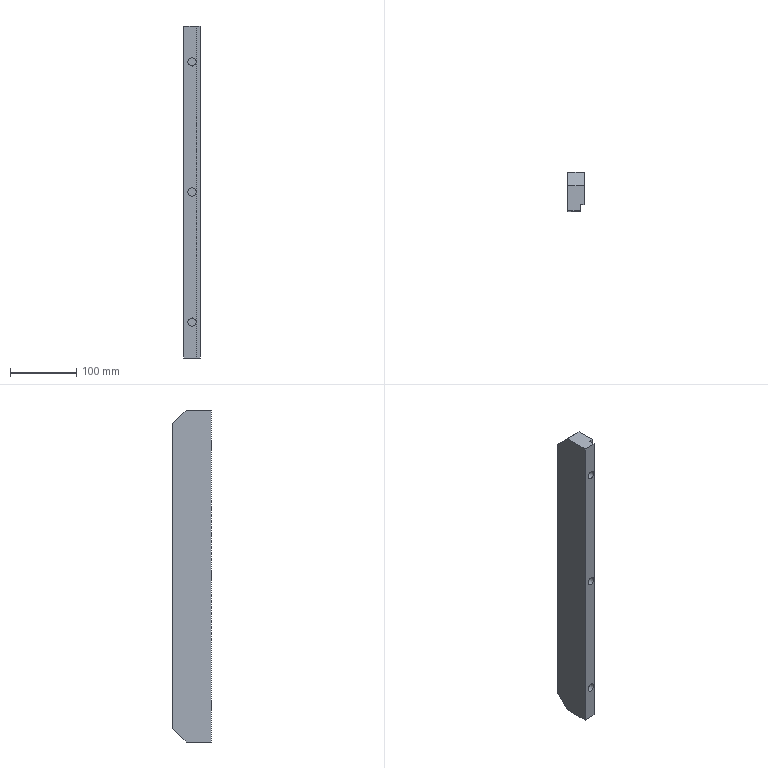NC program | NX | posted with a generic post | part box 25 x 58 x 500 mm
Whole program:
N10 G17 G21 G94 G90
(DRILLING , TOOL : ZXZ)
N12 T01 M6
N14 G54
N16 G17 G0 G90 X196. Y0. S3000 M3
N18 G43 Z30. H1
N20 G94 G81 G98 Z-1. F200. R3.
N22 X-196.
N24 X0.
N26 G80
N28 G0 X0. Y0. Z30.
N30 M5
N32 M2